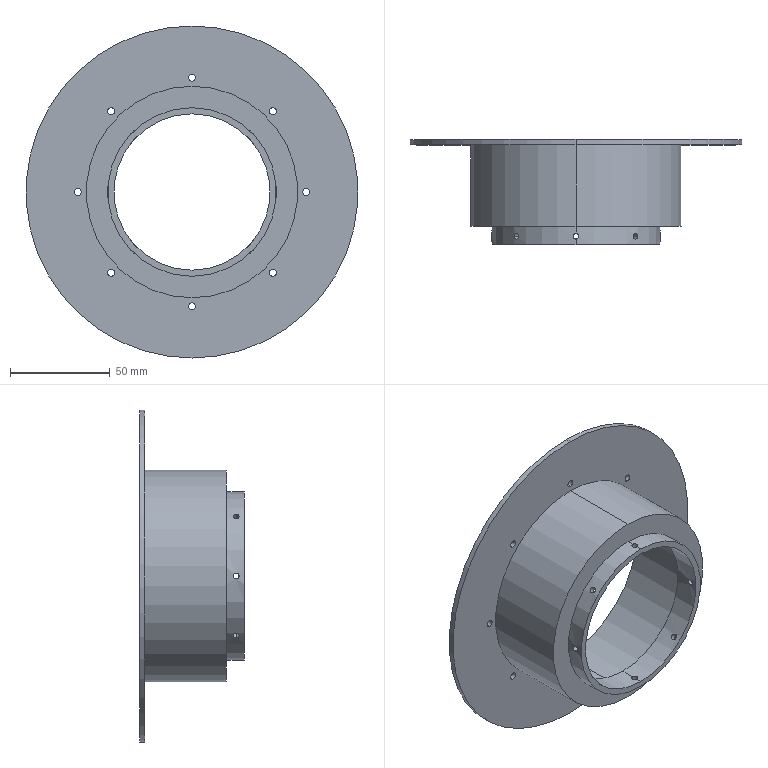Part | SolidWorks | features SavedExtBody 1 | 1 solid | 47 faces | box 166.652 x 52.651 x 166.652 mm | volume 97118 mm3 | cylinder 42 | plane 5 | commonest cylinder face diameters 3 x16 3.5 x16 78.435 x2 84.561 x2 99.754 x2 106.126 x2